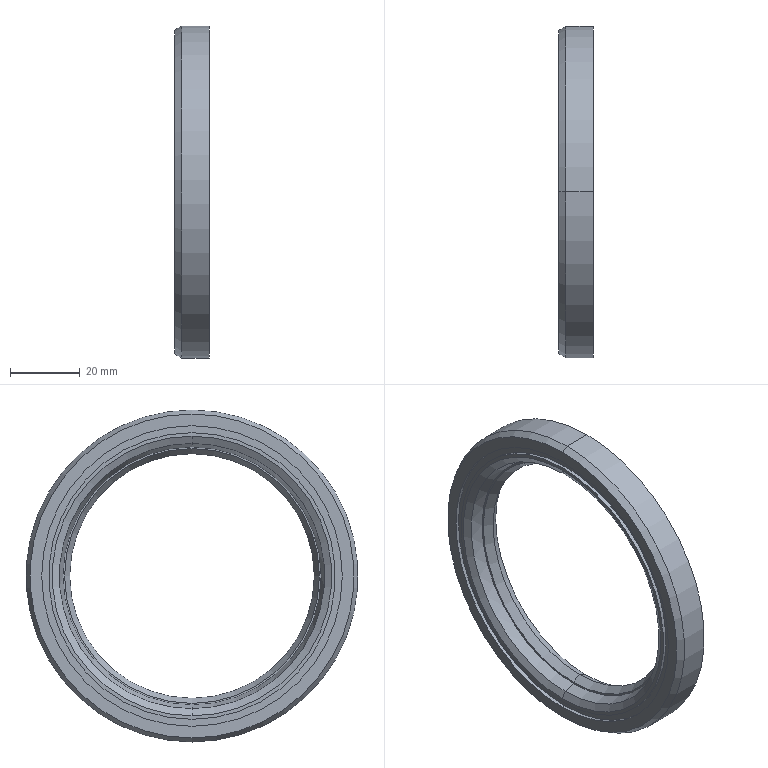Part | STEP file | SIMMERING_KORPUS1V11 | 1 solid | 50 faces | box 10 x 95 x 95 mm | volume 14984 mm3 | cylinder 16 | torus 14 | cone 10 | plane 10 | commonest cylinder face diameters 78.5 x2 82 x2 82.5 x2 86 x2 89 x2 91 x2